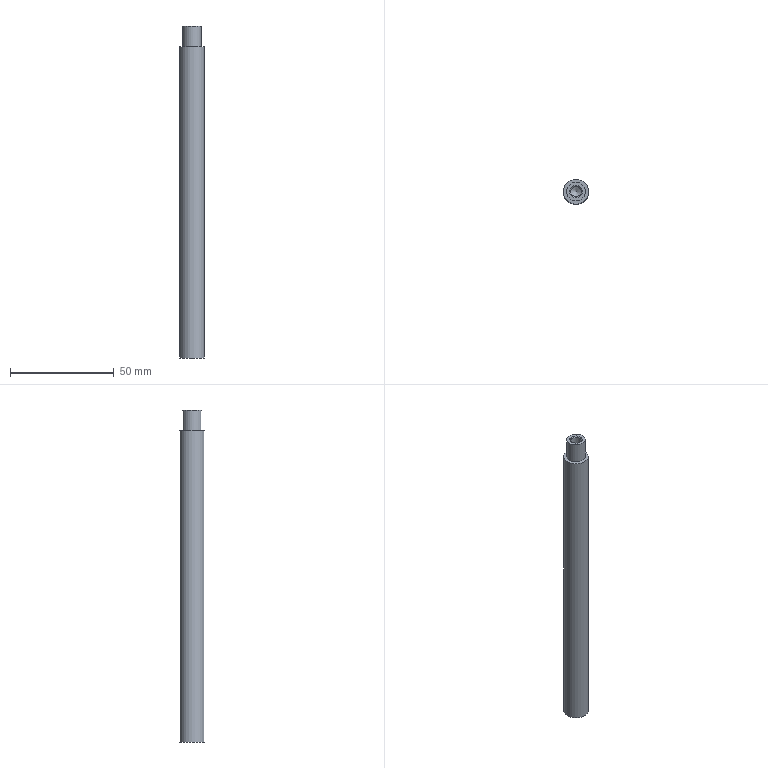Part | STEP file | 冲床-300配套压波_id770_x_t | 1 solid | 8 faces | box 12 x 12 x 160 mm | volume 17294 mm3 | cylinder 3 | plane 3 | cone 2 | commonest cylinder face diameters 5 x1 9 x1 12 x1
STEP:
#1=CARTESIAN_POINT('',(1754.,85.,53.));
#2=VERTEX_POINT('',#1);
#3=CARTESIAN_POINT('',(1760.,85.,53.));
#4=DIRECTION('',(0.,0.,1.));
#5=DIRECTION('',(-1.,0.,0.));
#6=AXIS2_PLACEMENT_3D('',#3,#4,#5);
#7=CIRCLE('',#6,6.);
#8=EDGE_CURVE('',#2,#2,#7,.T.);
#9=ORIENTED_EDGE('',*,*,#8,.T.);
#10=EDGE_LOOP('',(#9));
#11=FACE_BOUND('',#10,.T.);
#12=CARTESIAN_POINT('',(1766.,85.,203.));
#13=VERTEX_POINT('',#12);
#14=CARTESIAN_POINT('',(1760.,85.,203.));
#15=DIRECTION('',(0.,0.,-1.));
#16=DIRECTION('',(1.,0.,0.));
#17=AXIS2_PLACEMENT_3D('',#14,#15,#16);
#18=CIRCLE('',#17,6.);
#19=EDGE_CURVE('',#13,#13,#18,.T.);
#20=ORIENTED_EDGE('',*,*,#19,.T.);
#21=EDGE_LOOP('',(#20));
#22=FACE_BOUND('',#21,.T.);
#23=CARTESIAN_POINT('',(1760.,85.,-77.));
#24=DIRECTION('',(0.,0.,1.));
#25=DIRECTION('',(1.,0.,0.));
#26=AXIS2_PLACEMENT_3D('',#23,#24,#25);
#27=CYLINDRICAL_SURFACE('',#26,6.);
#28=ADVANCED_FACE('',(#11,#22),#27,.T.);
#29=ORIENTED_EDGE('',*,*,#8,.F.);
#30=EDGE_LOOP('',(#29));
#31=FACE_OUTER_BOUND('',#30,.T.);
#32=CARTESIAN_POINT('',(1805.,0.,53.));
#33=DIRECTION('',(0.,0.,-1.));
#34=DIRECTION('',(-1.,0.,0.));
#35=AXIS2_PLACEMENT_3D('',#32,#33,#34);
#36=PLANE('',#35);
#37=ADVANCED_FACE('',(#31),#36,.T.);
#38=ORIENTED_EDGE('',*,*,#19,.F.);
#39=EDGE_LOOP('',(#38));
#40=FACE_BOUND('',#39,.T.);
#41=CARTESIAN_POINT('',(1764.5,85.,203.));
#42=VERTEX_POINT('',#41);
#43=CARTESIAN_POINT('',(1760.,85.,203.));
#44=DIRECTION('',(0.,0.,-1.));
#45=DIRECTION('',(1.,0.,0.));
#46=AXIS2_PLACEMENT_3D('',#43,#44,#45);
#47=CIRCLE('',#46,4.5);
#48=EDGE_CURVE('',#42,#42,#47,.T.);
#49=ORIENTED_EDGE('',*,*,#48,.T.);
#50=EDGE_LOOP('',(#49));
#51=FACE_BOUND('',#50,.T.);
#52=CARTESIAN_POINT('',(60.,0.,203.));
#53=DIRECTION('',(0.,0.,1.));
#54=DIRECTION('',(1.,0.,0.));
#55=AXIS2_PLACEMENT_3D('',#52,#53,#54);
#56=PLANE('',#55);
#57=ADVANCED_FACE('',(#40,#51),#56,.T.);
#58=CARTESIAN_POINT('',(1764.5,85.,213.));
#59=VERTEX_POINT('',#58);
#60=CARTESIAN_POINT('',(1760.,85.,213.));
#61=DIRECTION('',(0.,0.,-1.));
#62=DIRECTION('',(1.,0.,0.));
#63=AXIS2_PLACEMENT_3D('',#60,#61,#62);
#64=CIRCLE('',#63,4.5);
#65=EDGE_CURVE('',#59,#59,#64,.T.);
#66=ORIENTED_EDGE('',*,*,#65,.T.);
#67=EDGE_LOOP('',(#66));
#68=FACE_BOUND('',#67,.T.);
#69=ORIENTED_EDGE('',*,*,#48,.F.);
#70=EDGE_LOOP('',(#69));
#71=FACE_BOUND('',#70,.T.);
#72=CARTESIAN_POINT('',(1760.,85.,-72.));
#73=DIRECTION('',(0.,0.,1.));
#74=DIRECTION('',(1.,0.,0.));
#75=AXIS2_PLACEMENT_3D('',#72,#73,#74);
#76=CYLINDRICAL_SURFACE('',#75,4.5);
#77=ADVANCED_FACE('',(#68,#71),#76,.T.);
#78=CARTESIAN_POINT('',(1763.,85.,213.));
#79=VERTEX_POINT('',#78);
#80=CARTESIAN_POINT('',(1760.,85.,213.));
#81=DIRECTION('',(0.,0.,-1.));
#82=DIRECTION('',(1.,0.,0.));
#83=AXIS2_PLACEMENT_3D('',#80,#81,#82);
#84=CIRCLE('',#83,3.);
#85=EDGE_CURVE('',#79,#79,#84,.T.);
#86=ORIENTED_EDGE('',*,*,#85,.T.);
#87=EDGE_LOOP('',(#86));
#88=FACE_BOUND('',#87,.T.);
#89=ORIENTED_EDGE('',*,*,#65,.F.);
#90=EDGE_LOOP('',(#89));
#91=FACE_BOUND('',#90,.T.);
#92=CARTESIAN_POINT('',(1805.,0.,213.));
#93=DIRECTION('',(0.,0.,1.));
#94=DIRECTION('',(1.,0.,0.));
#95=AXIS2_PLACEMENT_3D('',#92,#93,#94);
#96=PLANE('',#95);
#97=ADVANCED_FACE('',(#88,#91),#96,.T.);
#98=CARTESIAN_POINT('',(1757.5,85.,198.));
#99=VERTEX_POINT('',#98);
#100=CARTESIAN_POINT('',(1760.,85.,198.));
#101=DIRECTION('',(0.,0.,1.));
#102=DIRECTION('',(-1.,0.,0.));
#103=AXIS2_PLACEMENT_3D('',#100,#101,#102);
#104=CIRCLE('',#103,2.5);
#105=EDGE_CURVE('',#99,#99,#104,.T.);
#106=ORIENTED_EDGE('',*,*,#105,.T.);
#107=EDGE_LOOP('',(#106));
#108=FACE_BOUND('',#107,.T.);
#109=CARTESIAN_POINT('',(1760.,85.,196.498));
#110=VERTEX_POINT('',#109);
#111=VERTEX_LOOP('',#110);
#112=FACE_BOUND('',#111,.T.);
#113=CARTESIAN_POINT('',(1760.,85.,198.));
#114=DIRECTION('',(0.,0.,1.));
#115=DIRECTION('',(1.,0.,0.));
#116=AXIS2_PLACEMENT_3D('',#113,#114,#115);
#117=CONICAL_SURFACE('',#116,2.5,59.);
#118=ADVANCED_FACE('',(#108,#112),#117,.F.);
#119=CARTESIAN_POINT('',(1762.5,85.,212.5));
#120=VERTEX_POINT('',#119);
#121=CARTESIAN_POINT('',(1760.,85.,212.5));
#122=DIRECTION('',(0.,0.,1.));
#123=DIRECTION('',(1.,0.,0.));
#124=AXIS2_PLACEMENT_3D('',#121,#122,#123);
#125=CIRCLE('',#124,2.5);
#126=EDGE_CURVE('',#120,#120,#125,.T.);
#127=ORIENTED_EDGE('',*,*,#126,.T.);
#128=EDGE_LOOP('',(#127));
#129=FACE_BOUND('',#128,.T.);
#130=ORIENTED_EDGE('',*,*,#105,.F.);
#131=EDGE_LOOP('',(#130));
#132=FACE_BOUND('',#131,.T.);
#133=CARTESIAN_POINT('',(1760.,85.,213.));
#134=DIRECTION('',(0.,0.,-1.));
#135=DIRECTION('',(-1.,0.,0.));
#136=AXIS2_PLACEMENT_3D('',#133,#134,#135);
#137=CYLINDRICAL_SURFACE('',#136,2.5);
#138=ADVANCED_FACE('',(#129,#132),#137,.F.);
#139=ORIENTED_EDGE('',*,*,#126,.F.);
#140=EDGE_LOOP('',(#139));
#141=FACE_BOUND('',#140,.T.);
#142=ORIENTED_EDGE('',*,*,#85,.F.);
#143=EDGE_LOOP('',(#142));
#144=FACE_BOUND('',#143,.T.);
#145=CARTESIAN_POINT('',(1760.,85.,213.));
#146=DIRECTION('',(0.,0.,1.));
#147=DIRECTION('',(1.,0.,0.));
#148=AXIS2_PLACEMENT_3D('',#145,#146,#147);
#149=CONICAL_SURFACE('',#148,3.,45.);
#150=ADVANCED_FACE('',(#141,#144),#149,.F.);
#151=CLOSED_SHELL('',(#28,#37,#57,#77,#97,#118,#138,#150));
#152=MANIFOLD_SOLID_BREP('',#151);
#153=(LENGTH_UNIT()NAMED_UNIT(*)SI_UNIT(.MILLI.,.METRE.));
#154=UNCERTAINTY_MEASURE_WITH_UNIT(LENGTH_MEASURE(0.00002),#153,'','');
#155=(NAMED_UNIT(*)PLANE_ANGLE_UNIT()SI_UNIT($,.RADIAN.));
#156=PLANE_ANGLE_MEASURE_WITH_UNIT(PLANE_ANGLE_MEASURE(0.01745),#155);
#157=DIMENSIONAL_EXPONENTS(0.,0.,0.,0.,0.,0.,0.);
#158=(CONVERSION_BASED_UNIT('DEGREE',#156)NAMED_UNIT(#157)PLANE_ANGLE_UNIT());
#159=(NAMED_UNIT(*)SI_UNIT($,.STERADIAN.)SOLID_ANGLE_UNIT());
#160=(GEOMETRIC_REPRESENTATION_CONTEXT(3)GLOBAL_UNCERTAINTY_ASSIGNED_CONTEXT((#154))GLOBAL_UNIT_ASSIGNED_CONTEXT((#153,#158,#159))REPRESENTATION_CONTEXT('',''));
#161=ADVANCED_BREP_SHAPE_REPRESENTATION('',(#152),#160);